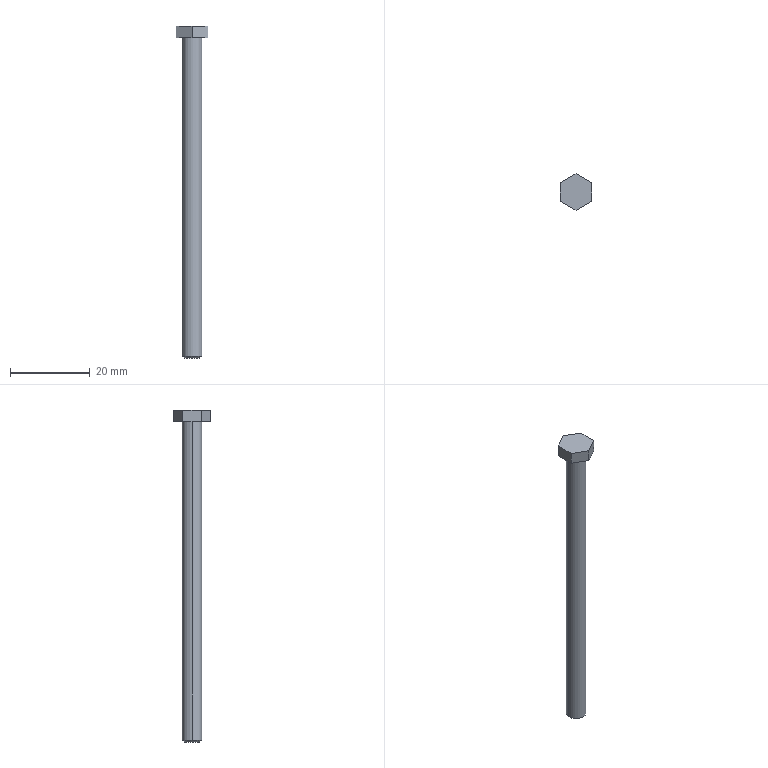Part | SolidWorks | features BaseBody 1 | 1 solid | 13 faces | box 8 x 9.238 x 83.5 mm | volume 1745 mm3 | plane 9 | cylinder 2 | cone 2 | commonest cylinder face diameters 5 x2
STEP:
#1=CARTESIAN_POINT('',(-2.5,0.,40.25));
#2=VERTEX_POINT('',#1);
#3=CARTESIAN_POINT('',(2.5,0.,40.25));
#4=VERTEX_POINT('',#3);
#5=CARTESIAN_POINT('',(0.,0.,40.25));
#6=DIRECTION('',(0.,0.,-1.));
#7=DIRECTION('',(-1.,0.,0.));
#8=AXIS2_PLACEMENT_3D('',#5,#6,#7);
#9=CIRCLE('',#8,2.5);
#10=EDGE_CURVE('',#2,#4,#9,.T.);
#11=ORIENTED_EDGE('',*,*,#10,.T.);
#12=CARTESIAN_POINT('',(2.5,0.,-39.75));
#13=VERTEX_POINT('',#12);
#14=CARTESIAN_POINT('',(2.5,0.,40.25));
#15=DIRECTION('',(0.,0.,-1.));
#16=VECTOR('',#15,1000.);
#17=LINE('',#14,#16);
#18=EDGE_CURVE('',#4,#13,#17,.T.);
#19=ORIENTED_EDGE('',*,*,#18,.T.);
#20=CARTESIAN_POINT('',(-2.5,0.,-39.75));
#21=VERTEX_POINT('',#20);
#22=CARTESIAN_POINT('',(0.,0.,-39.75));
#23=DIRECTION('',(0.,0.,1.));
#24=DIRECTION('',(-1.,0.,0.));
#25=AXIS2_PLACEMENT_3D('',#22,#23,#24);
#26=CIRCLE('',#25,2.5);
#27=EDGE_CURVE('',#13,#21,#26,.T.);
#28=ORIENTED_EDGE('',*,*,#27,.T.);
#29=CARTESIAN_POINT('',(-2.5,0.,40.25));
#30=DIRECTION('',(0.,0.,-1.));
#31=VECTOR('',#30,1000.);
#32=LINE('',#29,#31);
#33=EDGE_CURVE('',#2,#21,#32,.T.);
#34=ORIENTED_EDGE('',*,*,#33,.F.);
#35=EDGE_LOOP('',(#11,#19,#28,#34));
#36=FACE_OUTER_BOUND('',#35,.T.);
#37=CARTESIAN_POINT('',(0.,0.,40.25));
#38=DIRECTION('',(0.,0.,-1.));
#39=DIRECTION('',(-1.,0.,0.));
#40=AXIS2_PLACEMENT_3D('',#37,#38,#39);
#41=CYLINDRICAL_SURFACE('',#40,2.5);
#42=ADVANCED_FACE('',(#36),#41,.T.);
#43=CARTESIAN_POINT('',(2.,0.,-40.25));
#44=VERTEX_POINT('',#43);
#45=CARTESIAN_POINT('',(-2.,0.,-40.25));
#46=VERTEX_POINT('',#45);
#47=CARTESIAN_POINT('',(0.,0.,-40.25));
#48=DIRECTION('',(0.,0.,1.));
#49=DIRECTION('',(1.,0.,0.));
#50=AXIS2_PLACEMENT_3D('',#47,#48,#49);
#51=CIRCLE('',#50,2.);
#52=EDGE_CURVE('',#44,#46,#51,.T.);
#53=ORIENTED_EDGE('',*,*,#52,.T.);
#54=CARTESIAN_POINT('',(-2.5,0.,-39.75));
#55=DIRECTION('',(-0.7071,0.,0.7071));
#56=VECTOR('',#55,1000.);
#57=LINE('',#54,#56);
#58=EDGE_CURVE('',#46,#21,#57,.T.);
#59=ORIENTED_EDGE('',*,*,#58,.T.);
#60=ORIENTED_EDGE('',*,*,#27,.F.);
#61=CARTESIAN_POINT('',(2.5,0.,-39.75));
#62=DIRECTION('',(0.7071,0.,0.7071));
#63=VECTOR('',#62,1000.);
#64=LINE('',#61,#63);
#65=EDGE_CURVE('',#44,#13,#64,.T.);
#66=ORIENTED_EDGE('',*,*,#65,.F.);
#67=EDGE_LOOP('',(#53,#59,#60,#66));
#68=FACE_OUTER_BOUND('',#67,.T.);
#69=CARTESIAN_POINT('',(0.,0.,-39.75));
#70=DIRECTION('',(0.,0.,1.));
#71=DIRECTION('',(1.,0.,0.));
#72=AXIS2_PLACEMENT_3D('',#69,#70,#71);
#73=CONICAL_SURFACE('',#72,2.5,0.7854);
#74=ADVANCED_FACE('',(#68),#73,.T.);
#75=ORIENTED_EDGE('',*,*,#18,.F.);
#76=CARTESIAN_POINT('',(0.,0.,40.25));
#77=DIRECTION('',(0.,0.,-1.));
#78=DIRECTION('',(-1.,0.,0.));
#79=AXIS2_PLACEMENT_3D('',#76,#77,#78);
#80=CIRCLE('',#79,2.5);
#81=EDGE_CURVE('',#4,#2,#80,.T.);
#82=ORIENTED_EDGE('',*,*,#81,.T.);
#83=ORIENTED_EDGE('',*,*,#33,.T.);
#84=CARTESIAN_POINT('',(0.,0.,-39.75));
#85=DIRECTION('',(0.,0.,1.));
#86=DIRECTION('',(-1.,0.,0.));
#87=AXIS2_PLACEMENT_3D('',#84,#85,#86);
#88=CIRCLE('',#87,2.5);
#89=EDGE_CURVE('',#21,#13,#88,.T.);
#90=ORIENTED_EDGE('',*,*,#89,.T.);
#91=EDGE_LOOP('',(#75,#82,#83,#90));
#92=FACE_OUTER_BOUND('',#91,.T.);
#93=CARTESIAN_POINT('',(0.,0.,40.25));
#94=DIRECTION('',(0.,0.,-1.));
#95=DIRECTION('',(-1.,0.,0.));
#96=AXIS2_PLACEMENT_3D('',#93,#94,#95);
#97=CYLINDRICAL_SURFACE('',#96,2.5);
#98=ADVANCED_FACE('',(#92),#97,.T.);
#99=ORIENTED_EDGE('',*,*,#58,.F.);
#100=CARTESIAN_POINT('',(0.,0.,-40.25));
#101=DIRECTION('',(0.,0.,1.));
#102=DIRECTION('',(1.,0.,0.));
#103=AXIS2_PLACEMENT_3D('',#100,#101,#102);
#104=CIRCLE('',#103,2.);
#105=EDGE_CURVE('',#46,#44,#104,.T.);
#106=ORIENTED_EDGE('',*,*,#105,.T.);
#107=ORIENTED_EDGE('',*,*,#65,.T.);
#108=ORIENTED_EDGE('',*,*,#89,.F.);
#109=EDGE_LOOP('',(#99,#106,#107,#108));
#110=FACE_OUTER_BOUND('',#109,.T.);
#111=CARTESIAN_POINT('',(0.,0.,-39.75));
#112=DIRECTION('',(0.,0.,1.));
#113=DIRECTION('',(1.,0.,0.));
#114=AXIS2_PLACEMENT_3D('',#111,#112,#113);
#115=CONICAL_SURFACE('',#114,2.5,0.7854);
#116=ADVANCED_FACE('',(#110),#115,.T.);
#117=CARTESIAN_POINT('',(0.,-4.619,40.25));
#118=VERTEX_POINT('',#117);
#119=CARTESIAN_POINT('',(4.,-2.309,40.25));
#120=VERTEX_POINT('',#119);
#121=CARTESIAN_POINT('',(0.,-4.619,40.25));
#122=DIRECTION('',(0.866,0.5,0.));
#123=VECTOR('',#122,1000.);
#124=LINE('',#121,#123);
#125=EDGE_CURVE('',#118,#120,#124,.T.);
#126=ORIENTED_EDGE('',*,*,#125,.F.);
#127=CARTESIAN_POINT('',(-4.,-2.309,40.25));
#128=VERTEX_POINT('',#127);
#129=CARTESIAN_POINT('',(-4.,-2.309,40.25));
#130=DIRECTION('',(0.866,-0.5,0.));
#131=VECTOR('',#130,1000.);
#132=LINE('',#129,#131);
#133=EDGE_CURVE('',#128,#118,#132,.T.);
#134=ORIENTED_EDGE('',*,*,#133,.F.);
#135=CARTESIAN_POINT('',(-4.,2.309,40.25));
#136=VERTEX_POINT('',#135);
#137=CARTESIAN_POINT('',(-4.,0.,40.25));
#138=DIRECTION('',(0.,-1.,0.));
#139=VECTOR('',#138,1000.);
#140=LINE('',#137,#139);
#141=EDGE_CURVE('',#136,#128,#140,.T.);
#142=ORIENTED_EDGE('',*,*,#141,.F.);
#143=CARTESIAN_POINT('',(0.,4.619,40.25));
#144=VERTEX_POINT('',#143);
#145=CARTESIAN_POINT('',(0.,4.619,40.25));
#146=DIRECTION('',(-0.866,-0.5,0.));
#147=VECTOR('',#146,1000.);
#148=LINE('',#145,#147);
#149=EDGE_CURVE('',#144,#136,#148,.T.);
#150=ORIENTED_EDGE('',*,*,#149,.F.);
#151=CARTESIAN_POINT('',(4.,2.309,40.25));
#152=VERTEX_POINT('',#151);
#153=CARTESIAN_POINT('',(4.,2.309,40.25));
#154=DIRECTION('',(-0.866,0.5,0.));
#155=VECTOR('',#154,1000.);
#156=LINE('',#153,#155);
#157=EDGE_CURVE('',#152,#144,#156,.T.);
#158=ORIENTED_EDGE('',*,*,#157,.F.);
#159=CARTESIAN_POINT('',(4.,0.,40.25));
#160=DIRECTION('',(0.,1.,0.));
#161=VECTOR('',#160,1000.);
#162=LINE('',#159,#161);
#163=EDGE_CURVE('',#120,#152,#162,.T.);
#164=ORIENTED_EDGE('',*,*,#163,.F.);
#165=EDGE_LOOP('',(#126,#134,#142,#150,#158,#164));
#166=FACE_OUTER_BOUND('',#165,.T.);
#167=ORIENTED_EDGE('',*,*,#10,.F.);
#168=ORIENTED_EDGE('',*,*,#81,.F.);
#169=EDGE_LOOP('',(#167,#168));
#170=FACE_BOUND('',#169,.T.);
#171=CARTESIAN_POINT('',(0.,0.,40.25));
#172=DIRECTION('',(0.,0.,1.));
#173=DIRECTION('',(1.,0.,0.));
#174=AXIS2_PLACEMENT_3D('',#171,#172,#173);
#175=PLANE('',#174);
#176=ADVANCED_FACE('',(#166,#170),#175,.F.);
#177=ORIENTED_EDGE('',*,*,#52,.F.);
#178=ORIENTED_EDGE('',*,*,#105,.F.);
#179=EDGE_LOOP('',(#177,#178));
#180=FACE_OUTER_BOUND('',#179,.T.);
#181=CARTESIAN_POINT('',(0.,0.,-40.25));
#182=DIRECTION('',(0.,0.,1.));
#183=DIRECTION('',(1.,0.,0.));
#184=AXIS2_PLACEMENT_3D('',#181,#182,#183);
#185=PLANE('',#184);
#186=ADVANCED_FACE('',(#180),#185,.F.);
#187=CARTESIAN_POINT('',(4.,-2.309,43.25));
#188=VERTEX_POINT('',#187);
#189=CARTESIAN_POINT('',(4.,2.309,43.25));
#190=VERTEX_POINT('',#189);
#191=CARTESIAN_POINT('',(4.,-2.309,43.25));
#192=DIRECTION('',(0.,1.,0.));
#193=VECTOR('',#192,1000.);
#194=LINE('',#191,#193);
#195=EDGE_CURVE('',#188,#190,#194,.T.);
#196=ORIENTED_EDGE('',*,*,#195,.F.);
#197=CARTESIAN_POINT('',(4.,-2.309,43.25));
#198=DIRECTION('',(0.,0.,1.));
#199=VECTOR('',#198,1000.);
#200=LINE('',#197,#199);
#201=EDGE_CURVE('',#120,#188,#200,.T.);
#202=ORIENTED_EDGE('',*,*,#201,.F.);
#203=ORIENTED_EDGE('',*,*,#163,.T.);
#204=CARTESIAN_POINT('',(4.,2.309,43.25));
#205=DIRECTION('',(0.,0.,-1.));
#206=VECTOR('',#205,1000.);
#207=LINE('',#204,#206);
#208=EDGE_CURVE('',#190,#152,#207,.T.);
#209=ORIENTED_EDGE('',*,*,#208,.F.);
#210=EDGE_LOOP('',(#196,#202,#203,#209));
#211=FACE_OUTER_BOUND('',#210,.T.);
#212=CARTESIAN_POINT('',(4.,-2.309,43.25));
#213=DIRECTION('',(-1.,0.,0.));
#214=DIRECTION('',(0.,-1.,0.));
#215=AXIS2_PLACEMENT_3D('',#212,#213,#214);
#216=PLANE('',#215);
#217=ADVANCED_FACE('',(#211),#216,.F.);
#218=CARTESIAN_POINT('',(0.,-4.619,43.25));
#219=VERTEX_POINT('',#218);
#220=CARTESIAN_POINT('',(0.,-4.619,43.25));
#221=DIRECTION('',(0.866,0.5,0.));
#222=VECTOR('',#221,1000.);
#223=LINE('',#220,#222);
#224=EDGE_CURVE('',#219,#188,#223,.T.);
#225=ORIENTED_EDGE('',*,*,#224,.F.);
#226=CARTESIAN_POINT('',(0.,-4.619,43.25));
#227=DIRECTION('',(0.,0.,1.));
#228=VECTOR('',#227,1000.);
#229=LINE('',#226,#228);
#230=EDGE_CURVE('',#118,#219,#229,.T.);
#231=ORIENTED_EDGE('',*,*,#230,.F.);
#232=ORIENTED_EDGE('',*,*,#125,.T.);
#233=ORIENTED_EDGE('',*,*,#201,.T.);
#234=EDGE_LOOP('',(#225,#231,#232,#233));
#235=FACE_OUTER_BOUND('',#234,.T.);
#236=CARTESIAN_POINT('',(0.,-4.619,43.25));
#237=DIRECTION('',(-0.5,0.866,0.));
#238=DIRECTION('',(-0.866,-0.5,0.));
#239=AXIS2_PLACEMENT_3D('',#236,#237,#238);
#240=PLANE('',#239);
#241=ADVANCED_FACE('',(#235),#240,.F.);
#242=CARTESIAN_POINT('',(-4.,-2.309,43.25));
#243=VERTEX_POINT('',#242);
#244=CARTESIAN_POINT('',(-4.,-2.309,43.25));
#245=DIRECTION('',(0.866,-0.5,0.));
#246=VECTOR('',#245,1000.);
#247=LINE('',#244,#246);
#248=EDGE_CURVE('',#243,#219,#247,.T.);
#249=ORIENTED_EDGE('',*,*,#248,.F.);
#250=CARTESIAN_POINT('',(-4.,-2.309,43.25));
#251=DIRECTION('',(0.,0.,1.));
#252=VECTOR('',#251,1000.);
#253=LINE('',#250,#252);
#254=EDGE_CURVE('',#128,#243,#253,.T.);
#255=ORIENTED_EDGE('',*,*,#254,.F.);
#256=ORIENTED_EDGE('',*,*,#133,.T.);
#257=ORIENTED_EDGE('',*,*,#230,.T.);
#258=EDGE_LOOP('',(#249,#255,#256,#257));
#259=FACE_OUTER_BOUND('',#258,.T.);
#260=CARTESIAN_POINT('',(-4.,-2.309,43.25));
#261=DIRECTION('',(0.5,0.866,0.));
#262=DIRECTION('',(-0.866,0.5,0.));
#263=AXIS2_PLACEMENT_3D('',#260,#261,#262);
#264=PLANE('',#263);
#265=ADVANCED_FACE('',(#259),#264,.F.);
#266=CARTESIAN_POINT('',(-4.,2.309,43.25));
#267=VERTEX_POINT('',#266);
#268=CARTESIAN_POINT('',(-4.,2.309,43.25));
#269=DIRECTION('',(0.,-1.,0.));
#270=VECTOR('',#269,1000.);
#271=LINE('',#268,#270);
#272=EDGE_CURVE('',#267,#243,#271,.T.);
#273=ORIENTED_EDGE('',*,*,#272,.F.);
#274=CARTESIAN_POINT('',(-4.,2.309,43.25));
#275=DIRECTION('',(0.,0.,1.));
#276=VECTOR('',#275,1000.);
#277=LINE('',#274,#276);
#278=EDGE_CURVE('',#136,#267,#277,.T.);
#279=ORIENTED_EDGE('',*,*,#278,.F.);
#280=ORIENTED_EDGE('',*,*,#141,.T.);
#281=ORIENTED_EDGE('',*,*,#254,.T.);
#282=EDGE_LOOP('',(#273,#279,#280,#281));
#283=FACE_OUTER_BOUND('',#282,.T.);
#284=CARTESIAN_POINT('',(-4.,2.309,43.25));
#285=DIRECTION('',(1.,0.,0.));
#286=DIRECTION('',(0.,0.,-1.));
#287=AXIS2_PLACEMENT_3D('',#284,#285,#286);
#288=PLANE('',#287);
#289=ADVANCED_FACE('',(#283),#288,.F.);
#290=CARTESIAN_POINT('',(0.,4.619,43.25));
#291=VERTEX_POINT('',#290);
#292=CARTESIAN_POINT('',(0.,4.619,43.25));
#293=DIRECTION('',(-0.866,-0.5,0.));
#294=VECTOR('',#293,1000.);
#295=LINE('',#292,#294);
#296=EDGE_CURVE('',#291,#267,#295,.T.);
#297=ORIENTED_EDGE('',*,*,#296,.F.);
#298=CARTESIAN_POINT('',(0.,4.619,43.25));
#299=DIRECTION('',(0.,0.,1.));
#300=VECTOR('',#299,1000.);
#301=LINE('',#298,#300);
#302=EDGE_CURVE('',#144,#291,#301,.T.);
#303=ORIENTED_EDGE('',*,*,#302,.F.);
#304=ORIENTED_EDGE('',*,*,#149,.T.);
#305=ORIENTED_EDGE('',*,*,#278,.T.);
#306=EDGE_LOOP('',(#297,#303,#304,#305));
#307=FACE_OUTER_BOUND('',#306,.T.);
#308=CARTESIAN_POINT('',(0.,4.619,43.25));
#309=DIRECTION('',(0.5,-0.866,0.));
#310=DIRECTION('',(0.866,0.5,0.));
#311=AXIS2_PLACEMENT_3D('',#308,#309,#310);
#312=PLANE('',#311);
#313=ADVANCED_FACE('',(#307),#312,.F.);
#314=CARTESIAN_POINT('',(4.,2.309,43.25));
#315=DIRECTION('',(-0.866,0.5,0.));
#316=VECTOR('',#315,1000.);
#317=LINE('',#314,#316);
#318=EDGE_CURVE('',#190,#291,#317,.T.);
#319=ORIENTED_EDGE('',*,*,#318,.F.);
#320=ORIENTED_EDGE('',*,*,#208,.T.);
#321=ORIENTED_EDGE('',*,*,#157,.T.);
#322=ORIENTED_EDGE('',*,*,#302,.T.);
#323=EDGE_LOOP('',(#319,#320,#321,#322));
#324=FACE_OUTER_BOUND('',#323,.T.);
#325=CARTESIAN_POINT('',(4.,2.309,43.25));
#326=DIRECTION('',(-0.5,-0.866,0.));
#327=DIRECTION('',(0.866,-0.5,0.));
#328=AXIS2_PLACEMENT_3D('',#325,#326,#327);
#329=PLANE('',#328);
#330=ADVANCED_FACE('',(#324),#329,.F.);
#331=ORIENTED_EDGE('',*,*,#272,.T.);
#332=ORIENTED_EDGE('',*,*,#248,.T.);
#333=ORIENTED_EDGE('',*,*,#224,.T.);
#334=ORIENTED_EDGE('',*,*,#195,.T.);
#335=ORIENTED_EDGE('',*,*,#318,.T.);
#336=ORIENTED_EDGE('',*,*,#296,.T.);
#337=EDGE_LOOP('',(#331,#332,#333,#334,#335,#336));
#338=FACE_OUTER_BOUND('',#337,.T.);
#339=CARTESIAN_POINT('',(0.,0.,43.25));
#340=DIRECTION('',(0.,0.,1.));
#341=DIRECTION('',(1.,0.,0.));
#342=AXIS2_PLACEMENT_3D('',#339,#340,#341);
#343=PLANE('',#342);
#344=ADVANCED_FACE('',(#338),#343,.T.);
#345=CLOSED_SHELL('',(#42,#74,#98,#116,#176,#186,#217,#241,#265,#289,#313,#330,#344));
#346=MANIFOLD_SOLID_BREP('',#345);
#347=CARTESIAN_POINT('',(0.,0.,0.));
#348=DIRECTION('',(0.,0.,1.));
#349=DIRECTION('',(1.,0.,0.));
#350=AXIS2_PLACEMENT_3D('',#347,#348,#349);
#351=(LENGTH_UNIT()NAMED_UNIT(*)SI_UNIT(.MILLI.,.METRE.));
#352=UNCERTAINTY_MEASURE_WITH_UNIT(LENGTH_MEASURE(0.00001),#351,'','');
#353=(NAMED_UNIT(*)PLANE_ANGLE_UNIT()SI_UNIT($,.RADIAN.));
#354=(NAMED_UNIT(*)SI_UNIT($,.STERADIAN.)SOLID_ANGLE_UNIT());
#355=(GEOMETRIC_REPRESENTATION_CONTEXT(3)GLOBAL_UNCERTAINTY_ASSIGNED_CONTEXT((#352))GLOBAL_UNIT_ASSIGNED_CONTEXT((#351,#353,#354))REPRESENTATION_CONTEXT('',''));
#356=ADVANCED_BREP_SHAPE_REPRESENTATION('',(#346,#350),#355);